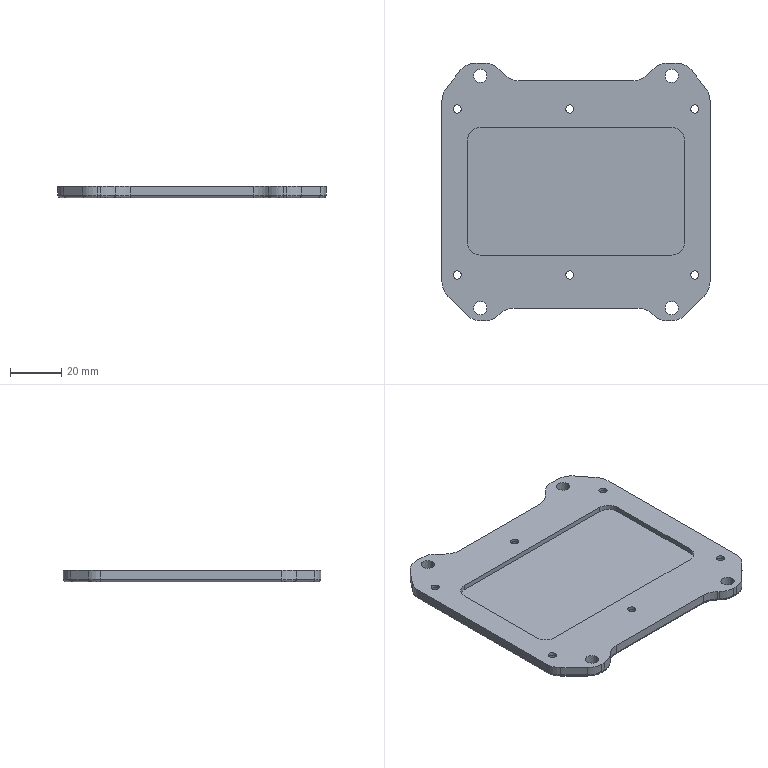CAM job | NX | 3-axis milling, drilling | part box 105 x 101 x 4.5 mm | stock box 125 x 125 x 4.5 mm
Tools:
number,name,description,diameter,corner_radius,flute_length,length,flutes
4,D4-12-D4-50-3T-FINISH,D4-12-D4-50-3T,4.0,0.0,12.0,50.0,3
3,D8-25-D8-60-3T-FINISH,D8-25-D8-60-3T,8.0,0.0,25.0,60.0,3
2,D8-24-D8-60波刀,D8*24*D8*60波刀,8.0,0.0,24.0,60.0,2
1,D80面刀,D80面刀,80.0,0.0,30.0,30.0,5
7,钻头D3.3-45-73,钻刀D3.3-45-73,3.3,0.0,45.0,73.0,2
5,倒角D8-90度,倒角D8-90度,8.0,0.0,8.0,60.0,2
8,球刀R1-4-D4-50,球刀R1-4-D4-50,2.0,1.0,4.0,4.5,2
Operations:
program,operation,operation_type,tool,method,geometry_group,spindle_rpm,surface_speed,feed_per_tooth,feed_cut,feed_plunge,cut_length_mm,path_length_mm,cut_time_min,machine_time_min
A1,FLOOR_WALL,VolumeBased25DMillingOperation,D80面刀,METHOD,WORKPIECE_54,3500.0,692.0,0.0571,800.0,100.0,390.0,652.756,0.4875,0.5138
A2,ADAPTIVE_MILLING,CavityMilling,D8-24-D8-60波刀,METHOD,WORKPIECE_54,5500.0,138.0,0.2273,2500.0,100.0,6798.208,6843.208,2.654,2.658
A3,SPOT_DRILLING,HoleDrilling,倒角D8-90度,METHOD,WORKPIECE_54,1600.0,40.0,0.0625,200.0,100.0,74.25,701.287,0.3712,0.434
A4,SPOT_DRILLING_1,HoleDrilling,钻头D3.3-45-73,METHOD,WORKPIECE_54,2500.0,25.0,0.04,200.0,100.0,108.0,563.0,0.54,0.5855
A5,PLANAR_MILL_1,PlanarMilling,D4-12-D4-50-3T-FINISH,METHOD,WORKPIECE_54,4500.0,56.0,0.037,500.0,100.0,700.715,1206.455,1.401,1.452
A5,PLANAR_MILL_1_COPY,PlanarMilling,D4-12-D4-50-3T-FINISH,METHOD,WORKPIECE_54,4500.0,56.0,0.037,500.0,100.0,707.282,1126.722,1.415,1.456
A7,PLANAR_MILL,PlanarMilling,D8-25-D8-60-3T-FINISH,METHOD,WORKPIECE_54,3500.0,87.0,0.0762,800.0,100.0,428.184,473.184,0.5352,0.5397
A8,CURVE_DRIVE,SurfaceContour,球刀R1-4-D4-50,METHOD,WORKPIECE_54,4500.0,28.0,0.2778,2500.0,100.0,15677.286,15711.711,6.271,6.274
B1,FLOOR_WALL_1,VolumeBased25DMillingOperation,D80面刀,METHOD,WORKPIECE_55,3500.0,692.0,0.0714,1000.0,100.0,1970.0,4043.466,1.97,2.177
B1,FLOOR_WALL_1_COPY,VolumeBased25DMillingOperation,D80面刀,METHOD,WORKPIECE_55,3500.0,692.0,0.0714,1000.0,100.0,394.0,659.185,0.394,0.4205
B2,PLANAR_MILL_2,PlanarMilling,D8-24-D8-60波刀,METHOD,WORKPIECE_55,4500.0,113.0,0.1667,1500.0,100.0,1407.893,1520.602,0.9386,0.9499
B3,PLANAR_MILL_2_COPY,PlanarMilling,D8-25-D8-60-3T-FINISH,METHOD,WORKPIECE_55,3500.0,87.0,0.0762,800.0,100.0,731.58,772.58,0.9145,0.9186
B4,PLANAR_MILL_3,PlanarMilling,倒角D8-90度,METHOD,WORKPIECE_55,3500.0,87.0,0.1429,1000.0,100.0,269.416,307.416,0.2694,0.2732
B4,PLANAR_MILL_3_COPY,PlanarMilling,倒角D8-90度,METHOD,WORKPIECE_55,3500.0,87.0,0.1429,1000.0,100.0,412.498,448.498,0.4125,0.4161
B4,SPOT_DRILLING_2,HoleDrilling,倒角D8-90度,METHOD,WORKPIECE_55,2500.0,62.0,0.04,200.0,100.0,102.0,1012.518,0.51,0.6011